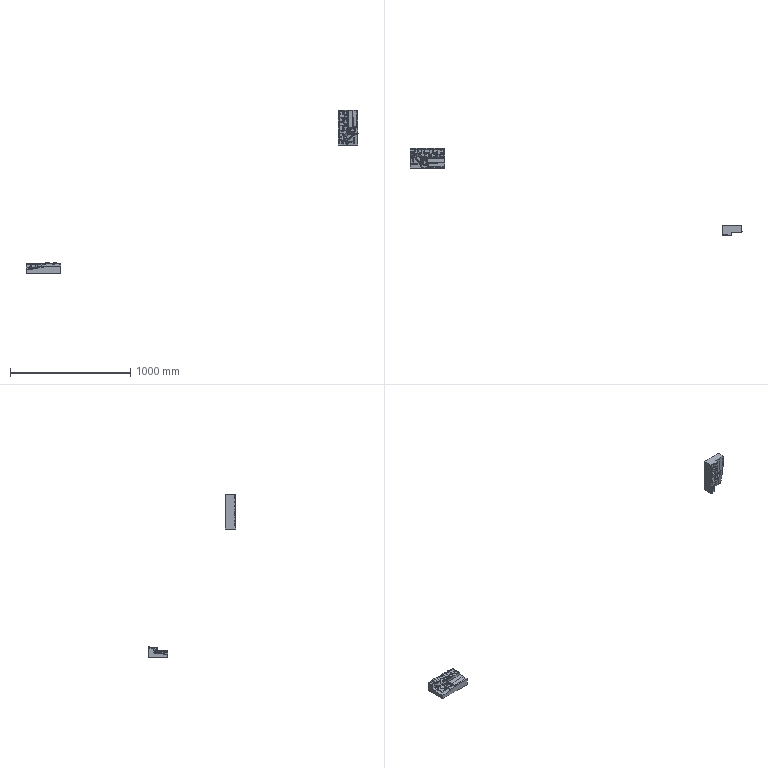NC program | NX | posted with a generic post | part box 2756 x 729.572 x 1353 mm
Lines 1 to 918 of 180527:
N10 G17 G21 G94 G90
(CAVITY_MILL , TOOL : D30R5)
N12 T00 M6
N14 G54
N16 G17 G0 G90 X96.082 Y-15. B0. C0. S3000 M3
N18 G43 Z10. H0
N20 Z-0.377
N22 G94 G1 Z-0.577 F2500.
N24 Y79.168
N26 X110.206
N28 G3 X111.586 Y83.525 R2.4
N30 G2 X109.837 Y84.788 R89.6
N32 G3 X108.189 Y85.332 R2.8
N34 G1 X81.958
N36 G3 X79.168 Y82.542 R2.8
N38 G1 Y81.958
N40 G3 X81.958 Y79.168 R2.8
N42 G1 X87.926
N44 G2 X90.753 Y77.997 R4.
N46 G1 X101.411 Y67.339
N48 G3 X104.239 Y66.168 R4.
N50 G1 X131.939
N52 G3 X133.985 Y67.016 R2.892
N54 G1 X136.507 Y69.538
N56 G2 X137.959 Y70.466 R4.
N58 G3 X137.288 Y80.049 R5.
N60 G1 X118.484 Y84.085
N62 G3 X112.546 Y80.246 R5.
N64 X116.386 Y74.308 R5.
N66 G1 X132.215 Y70.91
N68 G2 X133.844 Y69.965 R3.043
N70 G1 X136.049 Y67.5
N72 G3 X139.03 Y66.168 R4.
N74 G1 X216.344
N76 G3 X220.332 Y70.156 R4.
N78 G1 Y75.916
N80 G3 X216.903 Y79.864 R4.
N82 G2 X209.985 Y81.159 R78.298
N84 G3 X208.148 Y81.151 R4.
N86 G2 X187.561 Y78.856 R80.961
N88 X156.417 Y80.486 R433.583
N90 X114.741 Y97.439 R76.6
N92 G3 X112.232 Y98.332 R4.
N94 G1 X70.156
N96 G3 X66.168 Y94.344 R4.
N98 G1 Y70.156
N100 G3 X70.156 Y66.168 R4.
N102 G1 X87.926
N104 G2 X90.753 Y64.997 R4.
N106 G1 X101.411 Y54.339
N108 G3 X104.239 Y53.168 R4.
N110 G1 X229.343
N112 G3 X233.332 Y57.157 R4.
N114 G1 Y88.099
N116 G3 X229.361 Y92.088 R4.
N118 G1 X227.394 Y92.097
N120 G2 X210.104 Y94.552 R65.298
N122 G3 X207.922 Y94.543 R4.
N124 G2 X187.78 Y91.855 R67.961
N126 X157.563 Y93.435 R420.583
N128 X119.802 Y110.266 R63.6
N130 G3 X117.094 Y111.332 R4.
N132 G1 X57.157
N134 G3 X53.168 Y107.343 R4.
N136 G1 Y57.157
N138 G3 X57.157 Y53.168 R4.
N140 G1 X87.926
N142 G2 X90.753 Y51.997 R4.
N144 G1 X101.411 Y41.339
N146 G3 X104.239 Y40.168 R4.
N148 G1 X242.342
N150 G3 X246.332 Y44.158 R4.
N152 G1 Y101.503
N154 G3 X242.214 Y105.491 R4.
N156 G1 X229.605 Y105.087
N158 X227.469 Y105.096
N160 G2 X210.315 Y108.121 R52.298
N162 G3 X207.635 Y108.115 R4.
N164 G2 X187.999 Y104.853 R54.961
N166 X158.709 Y106.385 R407.583
N168 X125.493 Y123.01 R50.6
N170 G3 X122.532 Y124.332 R4.
N172 G1 X44.158
N174 G3 X40.168 Y120.342 R4.
N176 G1 Y44.158
N178 G3 X44.158 Y40.168 R4.
N180 G1 X87.926
N182 G2 X90.753 Y38.997 R4.
N184 G1 X101.411 Y28.339
N186 G3 X104.239 Y27.168 R4.
N188 G1 X255.342
N190 G3 X259.332 Y31.159 R4.
N192 G1 Y114.93
N194 G3 X255.092 Y118.914 R4.
N196 G1 X254.963 Y118.906
N198 X229.426 Y118.088
N200 X227.547 Y118.096
N202 G2 X210.703 Y122.031 R39.298
N204 G3 X207.234 Y122.033 R4.
N206 G2 X188.218 Y117.851 R41.961
N208 X159.854 Y119.334 R394.583
N210 X132.11 Y135.595 R37.6
N212 G3 X128.821 Y137.332 R4.
N214 G1 X31.159
N216 G3 X27.168 Y133.341 R4.
N218 G1 Y31.159
N220 G3 X31.159 Y27.168 R4.
N222 G1 X87.927
N224 G2 X90.753 Y25.997 R4.
N226 G1 X101.411 Y15.339
N228 G3 X104.239 Y14.168 R4.
N230 G1 X268.34
N232 G3 X272.332 Y18.16 R4.
N234 G1 Y131.544
N236 G3 X266.405 Y135.041 R4.
N238 G2 X255.95 Y131.993 R24.829
N240 G1 X254.348 Y131.893
N242 X229.246 Y131.089
N244 X227.629 Y131.096
N246 G2 X211.478 Y136.81 R26.298
N248 G3 X206.519 Y136.815 R4.
N250 G2 X203.506 Y134.763 R25.432
N252 X188.44 Y130.849 R28.961
N254 X161. Y132.284 R381.583
N256 X140.268 Y147.802 R24.6
N258 G3 X136.556 Y150.332 R4.
N260 G1 X18.16
N262 G3 X14.168 Y146.34 R4.
N264 G1 Y18.16
N266 G3 X18.16 Y14.168 R4.
N268 G1 X87.927
N270 G2 X90.753 Y12.997 R4.
N272 G1 X101.411 Y2.339
N274 G3 X104.239 Y1.168 R4.
N276 G1 X285.325
N278 X285.332 Y1.175
N280 Y163.325
N282 X285.325 Y163.332
N284 X277.317
N286 G3 X276.312 Y162.544 R1.035
N288 G1 X276.257 Y162.322
N290 G2 X274.203 Y159.827 R3.729
N292 G3 X271.408 Y156.302 R5.
N294 G1 X268.168 Y140.633
N296 G3 X272.052 Y134.724 R5.
N298 X277.961 Y138.608 R5.
N300 G1 X281.201 Y154.277
N302 G3 X279.47 Y159.159 R5.
N304 G2 X278.677 Y160.628 R2.198
N306 G1 X278.504 Y162.264
N308 G3 X277.317 Y163.332 R1.194
N310 G1 X267.447
N312 G3 X266.276 Y160.701 R4.
N314 G1 X265.962 Y154.284
N316 G2 X255.137 Y144.967 R11.829
N318 G1 X253.734 Y144.88
N320 X229.066 Y144.09
N322 X227.719 Y144.096
N324 G2 X214.917 Y154.284 R13.298
N326 G1 X214.732 Y155.628
N328 X214.716 Y160.518
N330 G3 X213.54 Y163.332 R4.
N332 G1 X204.354
N334 G3 X203.179 Y160.506 R4.
N336 G1 X203.178 Y156.971
N338 X203.157 Y156.337
N340 G2 X196.976 Y146.004 R12.432
N342 X188.663 Y143.847 R15.961
N344 X162.146 Y145.233 R368.583
N346 X151.57 Y156.571 R11.6
N348 G3 X151.615 Y157.164 R4.
N350 G1 Y158.315
N352 X151.6 Y160.531
N354 G3 X150.425 Y163.332 R4.
N356 G1 X1.175
N358 X1.168 Y163.325
N360 Y1.175
N362 X1.175 Y1.168
N364 X111.082
N366 Y-15.
N368 Z-0.377
N370 G0 Z0.3
N372 X98.438
N374 Z-0.954
N376 G1 Z-1.154
N378 Y0.305
N380 X100.31 Y78.305
N382 X100.349 Y78.304
N384 X108.571
N386 G3 X109.952 Y82.661 R2.4
N388 G2 X107.161 Y84.706 R92.093
N390 G3 X103.374 Y84.762 R3.2
N392 G2 X99.865 Y82.366 R91.256
N394 G3 X98.841 Y78.859 R2.8
N396 G1 X103.939 Y67.648
N398 G3 X107.58 Y65.304 R4.
N400 G1 X130.088
N402 G3 X132.123 Y66.147 R2.881
N404 G1 X134.632 Y68.651
N406 G2 X136.094 Y69.581 R4.
N408 G3 X135.457 Y79.167 R5.
N410 G1 X116.864 Y83.222
N412 G3 X110.914 Y79.402 R5.
N414 X114.733 Y73.451 R5.
N416 G1 X130.365 Y70.042
N418 G2 X131.982 Y69.099 R3.036
N420 G1 X134.179 Y66.64
N422 G3 X137.162 Y65.304 R4.
N424 G1 X217.208
N426 G3 X221.196 Y69.292 R4.
N428 G1 Y74.929
N430 G3 X217.713 Y78.883 R4.
N432 G2 X209.881 Y80.277 R80.509
N434 G3 X208.094 Y80.272 R4.
N436 G2 X187.608 Y78.062 R83.589
N438 X158.872 Y78.903 R1188.078
N440 G1 X155.904 Y79.168
N442 G2 X111.137 Y98.224 R79.093
N444 G3 X108.536 Y99.196 R4.
N446 G1 X102.191
N448 G3 X99.683 Y98.301 R4.
N450 G2 X68.363 Y82.795 R78.256
N452 G3 X65.305 Y78.92 R4.
N454 G1 X65.304 Y76.486
N456 G3 X66.287 Y74.411 R2.683
N458 G1 X69.002 Y72.189
N460 G2 X69.699 Y71.452 R4.
N462 G3 X74.683 Y69.488 R5.
N464 G1 X94.402 Y73.281
N466 G3 X98.368 Y79.135 R5.
N468 X92.513 Y83.101 R5.
N470 G1 X72.794 Y79.308
N472 G3 X68.931 Y75.772 R5.
N474 G2 X68.304 Y74.703 R2.48
N476 G1 X66.469 Y72.861
N478 G3 X65.304 Y70.04 R4.
N480 G1 Y69.292
N482 G3 X69.292 Y65.304 R4.
N484 G1 X90.282
N486 G2 X93.109 Y64.134 R4.
N488 G1 X103.766 Y53.476
N490 G3 X106.595 Y52.304 R4.
N492 G1 X230.207
N494 G3 X234.196 Y56.293 R4.
N496 G1 Y87.275
N498 G3 X230.148 Y91.263 R4.
N500 G1 X228.885 Y91.245
N502 G2 X210.014 Y93.647 R67.509
N504 G3 X207.904 Y93.643 R4.
N506 G2 X187.817 Y91.06 R70.589
N508 X159.716 Y91.88 R1175.078
N510 G1 X157.07 Y92.115
N512 G2 X116.428 Y111.042 R66.093
N514 G3 X113.629 Y112.196 R4.
N516 G1 X97.331
N518 G3 X94.627 Y111.132 R4.
N520 G2 X55.939 Y93.908 R65.256
N522 G3 X52.305 Y89.936 R4.
N524 G1 X52.304 Y56.293
N526 G3 X56.293 Y52.304 R4.
N528 G1 X90.282
N530 G2 X93.109 Y51.134 R4.
N532 G1 X103.766 Y40.476
N534 G3 X106.595 Y39.304 R4.
N536 G1 X243.206 Y39.305
N538 G3 X247.196 Y43.294 R4.
N540 G1 Y100.468
N542 G3 X243.147 Y104.457 R4.
N544 G1 X228.693 Y104.243
N546 G2 X210.234 Y107.176 R54.509
N548 G3 X207.66 Y107.174 R4.
N550 G2 X188.026 Y104.058 R57.589
N552 X160.558 Y104.856 R1162.078
N554 G1 X158.236 Y105.063
N556 G2 X122.356 Y123.778 R53.093
N558 G3 X119.312 Y125.196 R4.
N560 G1 X91.91
N562 G3 X88.959 Y123.885 R4.
N564 G2 X49.104 Y106.664 R52.256
N566 X43.558 Y106.724 R50.259
N568 G3 X39.305 Y102.743 R4.
N570 G1 X39.304 Y43.294
N572 G3 X43.294 Y39.304 R4.
N574 G1 X90.282
N576 G2 X93.109 Y38.134 R4.
N578 G1 X103.766 Y27.476
N580 G3 X106.595 Y26.304 R4.
N582 G1 X256.206 Y26.305
N584 G3 X260.196 Y30.295 R4.
N586 G1 Y113.805
N588 G3 X255.958 Y117.788 R4.
N590 G1 X254.465 Y117.695
N592 X248.763 Y117.541
N594 X228.501 Y117.242
N596 G2 X210.614 Y121.003 R41.509
N598 G3 X207.321 Y121.01 R4.
N600 G2 X188.235 Y117.057 R44.589
N602 X161.399 Y117.833 R1149.078
N604 G1 X159.396 Y118.011
N606 G2 X129.396 Y136.069 R40.093
N608 G1 X129.212 Y136.356
N610 G3 X125.855 Y138.196 R4.
N612 G1 X85.669
N614 G3 X82.401 Y136.489 R4.
N616 G2 X48.948 Y119.672 R39.256
N618 X31.903 Y122.757 R37.259
N620 G3 X26.305 Y119.1 R4.
N622 G1 X26.304 Y30.295
N624 G3 X30.295 Y26.304 R4.
N626 G1 X90.282
N628 G2 X93.109 Y25.134 R4.
N630 G1 X103.766 Y14.476
N632 G3 X106.595 Y13.305 R4.
N634 G1 X269.205
N636 G3 X273.196 Y17.296 R4.
N638 G1 Y130.415
N640 G3 X267.314 Y133.935 R4.
N642 G2 X256.995 Y130.878 R26.549
N644 G1 X253.886 Y130.684
N646 X248.492 Y130.539
N648 X228.309 Y130.241
N650 G2 X211.309 Y135.554 R28.509
N652 G3 X206.665 Y135.549 R4.
N654 G2 X203.193 Y133.443 R26.22
N656 X188.45 Y130.055 R31.589
N658 X162.238 Y130.809 R1136.078
N660 G1 X160.558 Y130.959
N662 G2 X140.291 Y143.161 R27.093
N664 X137.683 Y148.505 R24.237
N666 G3 X133.912 Y151.196 R4.
N668 G1 X78.066
N670 G3 X74.39 Y148.752 R4.
N672 G2 X49.006 Y132.679 R26.256
N674 G3 X48.569 Y132.673 R4.
N676 G2 X24.084 Y148.573 R24.259
N678 G3 X20.338 Y151.196 R4.
N680 G1 X17.296
N682 G3 X13.305 Y147.204 R4.
N684 G1 Y137.598
N686 G3 X14.313 Y135.488 R2.712
N688 G1 X16.734 Y133.534
N690 G2 X17.915 Y131.957 R4.
N692 G1 X20.798 Y125.016
N694 G3 X27.333 Y122.316 R5.
N696 X30.033 Y128.851 R5.
N698 G1 X26.081 Y138.366
N700 G3 X16.489 Y136.958 R5.
N702 G2 X15.892 Y135.616 R2.355
N704 G1 X14.302 Y133.862
N706 G3 X13.305 Y131.274 R3.854
N708 G1 Y17.296
N710 G3 X17.296 Y13.305 R4.
N712 G1 X90.282
N714 G2 X93.109 Y12.134 R4.
N716 G1 X103.766 Y1.476
N718 G3 X106.595 Y0.305 R4.
N720 G1 X284.031
N722 G3 X286.196 Y2.469 R4.
N724 G1 Y150.989
N726 G3 X285.2 Y152.257 R1.305
N728 G1 X284.428 Y152.445
N730 G2 X281.821 Y154.502 R4.
N732 G3 X272.527 Y153.444 R5.
N734 G1 X269.044 Y139.688
N736 G3 X272.663 Y133.614 R5.
N738 X278.738 Y137.234 R5.
N740 G1 X281.298 Y147.345
N742 G2 X283.485 Y149.326 R2.665
N744 G1 X284.954 Y149.547
N746 G3 X286.196 Y150.989 R1.458
N748 G1 Y162.031
N750 G3 X284.031 Y164.196 R4.
N752 G1 X270.638
N754 G3 X268.169 Y160.516 R4.
N756 G1 X268.156 Y155.628
N758 X267.971 Y154.284
N760 G2 X256.001 Y143.841 R13.549
N762 G1 X253.308 Y143.674
N764 X248.22 Y143.536
N766 X228.117 Y143.239
N768 G2 X217.129 Y147.577 R15.509
N770 X213.318 Y156.527 R12.444
N772 G1 X213.314 Y160.509
N774 G3 X210.845 Y164.196 R4.
N776 G1 X206.744
N778 G3 X204.593 Y160.905 R3.6
N780 G1 X204.595 Y156.971
N782 X204.591 Y156.678
N784 G2 X197.332 Y145.047 R13.22
N786 X188.663 Y143.053 R18.589
N788 X163.075 Y143.786 R1123.078
N790 G1 X162.402 Y143.846
N792 X161.728 Y143.906
N794 G2 X151.186 Y150.254 R14.093
N796 X149.367 Y156.381 R11.237
N798 G1 X149.366 Y160.506
N800 G3 X146.896 Y164.196 R4.
N802 G1 X65.7
N804 G3 X63.231 Y160.505 R4.
N806 G1 Y156.599
N808 G2 X49.011 Y145.704 R13.256
N810 G3 X48.2 Y145.692 R4.
N812 G2 X35.805 Y154.842 R11.259
N814 G1 X35.785 Y154.954
N816 X35.789 Y160.903
N818 G3 X33.638 Y164.196 R3.6
N820 G1 X2.469
N822 G3 X0.305 Y162.031 R4.
N824 G1 Y2.469
N826 G3 X2.469 Y0.305 R4.
N828 G1 X113.438
N830 Y-15.
N832 Z-0.954
N834 G0 Z-0.277
N836 X109.138
N838 Z-1.532
N840 G1 Z-1.732
N842 Y0.
N844 X109.902 Y78.
N846 X109.904
N848 X112.501
N850 G3 X112.924 Y79.476 R0.8
N852 G2 X111.658 Y80.279 R95.628
N854 G3 X110.812 Y80.286 R0.8
N856 G2 X109.494 Y79.484 R90.266
N858 G3 X109.138 Y78.587 R0.8
N860 G1 X114.561 Y67.271
N862 G3 X118.168 Y65. R4.
N864 G1 X128.596
N866 G3 X130.652 Y65.853 R2.905
N868 G1 X133.188 Y68.396
N870 G2 X134.629 Y69.321 R4.
N872 G3 X133.923 Y78.902 R5.
N874 G1 X119.29 Y81.989
N876 G3 X113.365 Y78.128 R5.
N878 X117.225 Y72.204 R5.
N880 G1 X128.869 Y69.748
N882 G2 X130.511 Y68.799 R3.05
N884 G1 X132.725 Y66.33
N886 G3 X135.704 Y65. R4.
N888 G1 X217.512
N890 G3 X221.5 Y68.988 R4.
N892 G1 Y74.267
N894 G3 X218. Y78.223 R4.
N896 G2 X209.849 Y79.639 R82.863
N898 G3 X208.097 Y79.635 R4.
N900 G2 X187.626 Y77.489 R84.885
N902 G1 X184.841 Y77.527
N904 X162.695 Y77.993
N906 X161.16 Y78.043
N908 G2 X118.109 Y91.591 R82.628
N910 X113.74 Y94.682 R77.9
N912 G3 X108.971 Y94.722 R4.
N914 G2 X91.919 Y85.247 R77.266
N916 X68.621 Y79.64 R83.261
N918 G3 X65. Y75.671 R4.
N920 G1 Y68.988
N922 G3 X68.988 Y65. R4.
N924 G1 X85.903
N926 G3 X88.191 Y66.015 R3.085
N928 G1 X90.517 Y68.587
N930 G2 X92.721 Y69.829 R4.
N932 G1 X105.086 Y72.226
N934 G3 X109.043 Y78.086 R5.
N936 X103.183 Y82.043 R5.
N938 G1 X87.458 Y78.995
N940 G3 X88.6 Y69.09 R5.
N942 G2 X90.308 Y68.778 R4.
N944 G1 X98.802 Y65.189
N946 G2 X99.639 Y64.709 R4.
N948 G1 X115.574 Y52.795
N950 G3 X117.966 Y52. R4.
N952 G1 X230.512
N954 G3 X234.5 Y55.988 R4.
N956 G1 Y86.63
N958 G3 X230.458 Y90.618 R4.
N960 G1 X229.291 Y90.602
N962 X227.152 Y90.613
N964 G2 X209.981 Y92.994 R69.863
N966 G3 X207.92 Y92.99 R4.
N968 G2 X187.827 Y90.487 R71.885
N970 G1 X185.067 Y90.525
N972 X163.04 Y90.989
N974 X161.551 Y91.037
N976 G2 X125.25 Y102.454 R69.628
N978 X114.502 Y111.306 R64.9
N980 G3 X111.663 Y112.5 R4.
N982 G1 X111.263
N984 G3 X108.467 Y111.349 R4.
N986 G2 X87.09 Y97.317 R64.266
N988 X64.595 Y92.382 R70.261
N990 G1 X62.355 Y92.288
N992 X55.905 Y92.154
N994 G3 X52. Y88.167 R4.
N996 G1 Y55.988
N998 G3 X55.988 Y52. R4.
N1000 G1 X100.983
N1002 G2 X103.809 Y50.829 R4.
N1004 G1 X114.467 Y40.172
N1006 G3 X117.295 Y39. R4.
N1008 G1 X243.511
N1010 G3 X247.5 Y42.989 R4.
N1012 G1 Y99.807
N1014 G3 X243.457 Y103.796 R4.
N1016 G1 X229.234 Y103.603
N1018 X227.277 Y103.612
N1020 G2 X210.189 Y106.497 R56.863
N1022 G3 X207.687 Y106.495 R4.
N1024 G2 X188.03 Y103.486 R58.885
N1026 G1 X185.293 Y103.523
N1028 X163.386 Y103.985
N1030 X161.939 Y104.031
N1032 G2 X132.39 Y113.317 R56.628
N1034 X120.563 Y124.026 R51.9
N1036 G3 X117.473 Y125.5 R4.
N1038 G1 X105.576
N1040 G3 X102.527 Y124.077 R4.
N1042 G2 X82.261 Y109.387 R51.266
N1044 X63.981 Y105.368 R57.261
N1046 G1 X61.947 Y105.282
N1048 X48.166 Y104.997
N1050 G2 X43.241 Y105.091 R55.915
N1052 G3 X39. Y101.11 R4.
N1054 G1 Y42.989
N1056 G3 X42.989 Y39. R4.
N1058 G1 X100.982
N1060 G2 X103.809 Y37.829 R4.
N1062 G1 X114.467 Y27.172
N1064 G3 X117.295 Y26. R4.
N1066 G1 X256.51
N1068 G3 X260.5 Y29.99 R4.
N1070 G1 Y113.029
N1072 G3 X256.31 Y117.015 R4.
N1074 G2 X255.367 Y116.978 R42.925
N1076 G1 X253.822 Y116.938
N1078 X229.178 Y116.603
N1080 X227.409 Y116.612
N1082 G2 X210.532 Y120.273 R43.863
N1084 G3 X207.357 Y120.276 R4.
N1086 G2 X188.236 Y116.484 R45.885
N1088 G1 X185.518 Y116.521
N1090 X163.731 Y116.98
N1092 X162.324 Y117.025
N1094 G2 X139.531 Y124.181 R43.628
N1096 X127.599 Y136.577 R38.9
N1098 G3 X124.191 Y138.5 R4.
N1100 G1 X98.996
N1102 G3 X95.625 Y136.636 R4.
N1104 G2 X77.432 Y121.457 R38.266
N1106 X63.36 Y118.353 R44.261
N1108 G1 X61.538 Y118.277
N1110 X47.868 Y117.993
N1112 G2 X31.421 Y120.821 R42.915
N1114 G3 X26. Y117.092 R4.
N1116 G1 Y29.99
N1118 G3 X29.99 Y26. R4.
N1120 G1 X100.983
N1122 G2 X103.809 Y24.829 R4.
N1124 G1 X114.467 Y14.172
N1126 G3 X117.295 Y13. R4.
N1128 G1 X269.508
N1130 G3 X273.5 Y16.992 R4.
N1132 G1 Y129.635
N1134 G3 X267.698 Y133.198 R4.
N1136 G2 X255.013 Y129.973 R29.925
N1138 G1 X253.565 Y129.935
N1140 X229.122 Y129.604
N1142 X227.554 Y129.611
N1144 G2 X211.499 Y134.443 R30.863
N1146 X211.159 Y134.664 R26.394
N1148 G3 X206.765 Y134.661 R4.
N1150 G2 X204.885 Y133.526 R26.556
N1152 X188.446 Y129.482 R32.885
N1154 G1 X185.744 Y129.519
N1156 X164.076 Y129.976
N1158 X162.704 Y130.02
N1160 G2 X146.672 Y135.044 R30.628
N1162 X136.248 Y148.736 R25.9
N1164 G3 X132.452 Y151.5 R4.
N1166 G1 X90.896
N1168 G3 X87.123 Y148.804 R4.
N1170 G2 X72.603 Y133.527 R25.266
N1172 X62.725 Y131.338 R31.261
N1174 G1 X61.13 Y131.271
N1176 X47.565 Y130.99
N1178 G2 X29.225 Y136.669 R29.915
N1180 X20.292 Y149.006 R24.428
N1182 G3 X16.874 Y151.5 R3.6
N1184 G1 X16.592
N1186 G3 X13. Y147.908 R3.6
N1188 G1 Y16.992
N1190 G3 X16.992 Y13. R4.
N1192 G1 X100.983
N1194 G2 X103.809 Y11.829 R4.
N1196 G1 X114.467 Y1.172
N1198 G3 X117.295 Y0. R4.
N1200 G1 X282.505
N1202 G3 X286.5 Y3.995 R4.
N1204 G1 Y148.788
N1206 G3 X285.548 Y150.011 R1.261
N1208 G1 X284.924 Y150.168
N1210 G2 X282.302 Y152.309 R4.
N1212 G3 X272.983 Y151.491 R5.
N1214 G1 X269.468 Y138.968
N1216 G3 X272.93 Y132.803 R5.
N1218 X279.096 Y136.265 R5.
N1220 G1 X281.621 Y145.261
N1222 G2 X283.788 Y147.156 R2.633
N1224 G1 X285.262 Y147.364
N1226 G3 X286.5 Y148.788 R1.438
N1228 G1 Y160.505
N1230 G3 X282.505 Y164.5 R4.
N1232 G1 X273.394
N1234 G3 X269.399 Y160.507 R4.
N1236 G1 X269.397 Y156.971
N1238 G2 X264.082 Y146.174 R13.143
N1240 X254.654 Y142.968 R16.925
N1242 G1 X253.308 Y142.933
N1244 X229.066 Y142.604
N1246 X227.719 Y142.611
N1248 G2 X218.486 Y145.406 R17.863
N1250 X212.295 Y156.359 R13.394
N1252 G1 X212.279 Y156.971
N1254 Y161.306
N1256 G3 X209.085 Y164.5 R3.2
N1258 G1 X208.873
N1260 G3 X205.679 Y161.304 R3.2
N1262 G1 X205.681 Y156.971
N1264 X205.67 Y156.496
N1266 G2 X198.635 Y144.925 R13.556
N1268 X188.663 Y142.481 R19.885
N1270 G1 X185.97 Y142.517
N1272 X164.422 Y142.972
N1274 X163.075 Y143.015
N1276 G2 X153.812 Y145.907 R17.628
N1278 X148.003 Y156.317 R12.9
N1280 G1 X147.984 Y156.971
N1282 X147.985 Y160.905
N1284 G3 X144.39 Y164.5 R3.6
N1286 G1 X78.996
N1288 G3 X75.402 Y160.826 R3.6
N1290 G1 X75.481 Y157.256
N1292 G2 X67.774 Y145.597 R12.266
N1294 X62.068 Y144.322 R18.261
N1296 G1 X60.721 Y144.265
N1298 X47.254 Y143.986
N1300 G2 X36.852 Y147.197 R16.915
N1302 X32.134 Y156.135 R11.428
N1304 G1 X32.111 Y156.971
N1306 X32.115 Y160.901
N1308 G3 X28.521 Y164.5 R3.6
N1310 G1 X3.995
N1312 G3 X0. Y160.505 R4.
N1314 G1 Y3.995
N1316 G3 X3.995 Y0. R4.
N1318 G1 X124.138
N1320 Y-15.
N1322 Z-1.532
N1324 G0 Z-0.854
N1326 X143.25
N1328 Z-2.109
N1330 G1 Z-2.309
N1332 Y65.
N1334 X217.512
N1336 G3 X221.5 Y68.988 R4.
N1338 G1 Y73.802
N1340 G3 X217.986 Y77.76 R4.
N1342 G2 X209.804 Y79.15 R84.079
N1344 G3 X208.107 Y79.151 R4.
N1346 G2 X188.006 Y77.085 R89.159
N1348 X161.74 Y77.474 R1970.402
N1350 X135.105 Y82.351 R84.447
N1352 G3 X132.815 Y82.462 R4.
N1354 G2 X98.315 Y81.769 R77.237
N1356 X91.823 Y83.196 R77.146
N1358 G3 X89.496 Y83.106 R4.
N1360 G2 X68.655 Y78.655 R84.131
N1362 G3 X65. Y74.682 R4.
N1364 G1 Y68.988
N1366 G3 X68.988 Y65. R4.
N1368 G1 X135.094
N1370 G2 X137.921 Y63.829 R4.
N1372 G1 X148.578 Y53.172
N1374 G3 X151.407 Y52. R4.
N1376 G1 X230.511
N1378 G3 X234.5 Y55.989 R4.
N1380 G1 Y86.186
N1382 G3 X230.471 Y90.175 R4.
N1384 G1 X229.224 Y90.162
N1386 X227.344 Y90.17
N1388 G2 X209.97 Y92.48 R71.079
N1390 G3 X207.981 Y92.483 R4.
N1392 G2 X207.324 Y92.317 R69.062
N1394 X188.132 Y90.085 R76.159
N1396 X162.01 Y90.471 R1957.402
N1398 X135.949 Y95.956 R71.447
N1400 G3 X133.238 Y96.08 R4.
N1402 G2 X100.761 Y94.539 R64.237
N1404 X91.531 Y96.84 R64.146
N1406 G3 X88.775 Y96.739 R4.
N1408 G2 X63.267 Y91.381 R71.131
N1410 G1 X61.704 Y91.345
N1412 X55.932 Y91.263
N1414 G3 X52. Y87.275 R4.
N1416 G1 Y55.989
N1418 G3 X55.989 Y52. R4.
N1420 G1 X135.094
N1422 G2 X137.92 Y50.829 R4.
N1424 G1 X148.578 Y40.172
N1426 G3 X151.407 Y39. R4.
N1428 G1 X243.511
N1430 G3 X247.5 Y42.989 R4.
N1432 G1 Y99.317
N1434 G3 X243.47 Y103.306 R4.
N1436 G1 X229.185 Y103.162
N1438 X227.429 Y103.169
N1440 G2 X210.197 Y105.948 R58.079
N1442 G3 X207.778 Y105.95 R4.
N1444 G2 X204.196 Y104.935 R56.062
N1446 X188.26 Y103.084 R63.159
N1448 X162.278 Y103.468 R1944.402
N1450 X136.846 Y109.856 R58.447
N1452 G3 X133.526 Y109.993 R4.
N1454 G2 X103.207 Y107.31 R51.237
N1456 X91.379 Y110.788 R51.146
N1458 G3 X88.002 Y110.681 R4.
N1460 G2 X62.966 Y104.378 R58.131
N1462 G1 X61.458 Y104.342
N1464 X49.408 Y104.171
N1466 X48.072 Y104.135
N1468 G2 X43.236 Y104.241 R60.832
N1470 G3 X39. Y100.259 R4.
N1472 G1 Y42.989
N1474 G3 X42.989 Y39. R4.
N1476 G1 X135.095
N1478 G2 X137.921 Y37.829 R4.
N1480 G1 X148.578 Y27.172
N1482 G3 X151.407 Y26. R4.
N1484 G1 X256.51
N1486 G3 X260.5 Y29.99 R4.
N1488 G1 Y112.49
N1490 G3 X256.325 Y116.476 R4.
N1492 G2 X255.157 Y116.437 R44.134
N1494 G1 X253.68 Y116.41
N1496 X229.145 Y116.163
N1498 X227.518 Y116.169
N1500 G2 X210.522 Y119.674 R45.079
N1502 G3 X207.44 Y119.671 R4.
N1504 G2 X201.069 Y117.553 R43.062
N1506 X188.39 Y116.084 R50.159
N1508 X162.546 Y116.465 R1931.402
N1510 X140.533 Y122.65 R45.447
N1512 X137.876 Y124.346 R39.513
N1514 G3 X133.567 Y124.502 R4.
N1516 G2 X105.653 Y120.083 R38.237
N1518 X91.484 Y125.36 R38.146
N1520 G3 X87.099 Y125.241 R4.
N1522 G2 X84.855 Y123.787 R38.327
N1524 X62.665 Y117.375 R45.131
N1526 G1 X61.213 Y117.34
N1528 X49.139 Y117.169
N1530 X47.786 Y117.132
N1532 G2 X31.302 Y119.77 R47.832
N1534 G3 X26. Y115.997 R4.
N1536 G1 Y29.99
N1538 G3 X29.99 Y26. R4.
N1540 G1 X135.095
N1542 G2 X137.92 Y24.83 R4.
N1544 G1 X148.578 Y14.172
N1546 G3 X151.407 Y13. R4.
N1548 G1 X269.508
N1550 G3 X273.5 Y16.992 R4.
N1552 G1 Y128.902
N1554 G3 X267.775 Y132.502 R4.
N1556 G2 X254.907 Y129.435 R31.134
N1558 G1 X253.494 Y129.409
N1560 X229.106 Y129.163
N1562 X227.613 Y129.169
N1564 G2 X211.801 Y133.531 R32.079
N1566 X211.064 Y133.977 R26.847
N1568 G3 X206.812 Y133.965 R4.
N1570 G2 X197.941 Y130.171 R30.062
N1572 X188.524 Y129.083 R37.159
N1574 X162.812 Y129.462 R1918.402
N1576 X147.084 Y133.879 R32.447
N1578 X139.358 Y140.708 R26.513
N1580 G3 X133.16 Y140.897 R4.
N1582 G2 X108.101 Y132.861 R25.237
N1584 X92.026 Y141.995 R25.146
N1586 G3 X85.678 Y141.83 R4.
N1588 G2 X78.17 Y134.937 R25.327
N1590 X62.366 Y130.371 R32.131
N1592 G1 X60.967 Y130.338
N1594 X48.87 Y130.166
N1596 X47.511 Y130.129
N1598 G2 X31.93 Y133.547 R34.832
N1600 X18.251 Y149.764 R25.833
N1602 G3 X15.952 Y151.5 R2.4
N1604 G1 X15.393
N1606 G3 X13. Y149.107 R2.4
N1608 G1 Y16.992
N1610 G3 X16.992 Y13. R4.
N1612 G1 X135.095
N1614 G2 X137.92 Y11.83 R4.
N1616 G1 X148.578 Y1.172
N1618 G3 X151.407 Y0. R4.
N1620 G1 X282.505
N1622 G3 X286.5 Y3.995 R4.
N1624 G1 Y146.969
N1626 G3 X285.588 Y148.149 R1.22
N1628 G1 X285.105 Y148.275
N1630 G2 X282.469 Y150.498 R4.
N1632 G3 X273.133 Y149.911 R5.
N1634 G1 X269.561 Y138.304
N1636 G3 X272.868 Y132.054 R5.
N1638 X279.118 Y135.362 R5.
N1640 G1 X281.639 Y143.552
N1642 G2 X283.787 Y145.366 R2.603
N1644 G1 X285.265 Y145.561
N1646 G3 X286.5 Y146.969 R1.42
N1648 G1 Y160.505
N1650 G3 X282.505 Y164.5 R4.
N1652 G1 X274.321
N1654 G3 X270.326 Y160.505 R4.
N1656 G1 X270.325 Y156.971
N1658 X270.316 Y156.455
N1660 G2 X264.116 Y145.324 R13.544
N1662 X254.654 Y142.433 R18.134
N1664 G1 X253.308 Y142.408
N1666 X229.066 Y142.163
N1668 X227.719 Y142.169
N1670 G2 X218.347 Y144.763 R19.079
N1672 X211.477 Y156.373 R13.847
N1674 G1 X211.462 Y156.971
N1676 X211.461 Y162.106
N1678 G3 X209.066 Y164.5 R2.4
N1680 G1 X208.949
N1682 G3 X206.554 Y162.104 R2.4
N1684 G1 X206.558 Y156.733
N1686 G2 X201.769 Y146.359 R13.613
N1688 X194.814 Y142.789 R17.062
N1690 X188.663 Y142.082 R24.159
N1692 X163.075 Y142.46 R1905.402
N1694 X153.636 Y145.107 R19.447
N1696 X146.94 Y156.364 R13.513
N1698 G1 X146.921 Y156.971
N1700 Y160.905
N1702 G3 X143.327 Y164.5 R3.6
N1704 G1 X138.11
N1706 X138.029 Y164.504
N1708 X138.007 Y164.426
N1710 G2 X137.672 Y164.161 R0.39
N1712 G3 X133.234 Y160.29 R5.
N1714 G1 X130.596 Y148.702
N1716 G3 X134.361 Y142.717 R5.
N1718 X140.346 Y146.482 R5.
N1720 G1 X142.985 Y158.07
N1722 G3 X138.414 Y164.171 R5.
N1724 G2 X138.236 Y164.322 R0.195
N1726 G1 X138.215 Y164.416
N1728 X138.217 Y164.478
N1730 X138.169 Y164.516
N1732 X138.11 Y164.5
N1734 X130.12
N1736 G3 X126.125 Y160.562 R4.
N1738 G1 X126.045 Y154.945
N1740 G2 X110.841 Y145.578 R12.237
N1742 G3 X110.252 Y145.691 R4.
N1744 G2 X99.526 Y156.606 R12.146
N1746 G1 Y160.505
N1748 G3 X95.531 Y164.5 R4.
N1750 G1 X81.484
N1752 G3 X77.489 Y160.507 R4.
N1754 G1 X77.488 Y157.629
N1756 G3 X77.818 Y157.214 R0.425
N1758 G2 X78.944 Y156.164 R1.54
N1760 G3 X80.47 Y153.832 R5.
N1762 G1 X88.948 Y146.556
N1764 G3 X95.998 Y147.094 R5.
N1766 X95.46 Y154.145 R5.
N1768 G1 X86.982 Y161.42
N1770 G3 X78.847 Y158.721 R5.
N1772 G2 X78.257 Y158.137 R0.77
N1774 G1 X77.824 Y158.044
N1776 G3 X77.488 Y157.629 R0.425
N1778 G1 X77.487 Y156.971
N1780 X77.468 Y156.299
N1782 G2 X71.485 Y146.086 R12.327
N1784 X62.068 Y143.368 R19.131
N1786 G1 X60.721 Y143.336
N1788 X48.601 Y143.164
N1790 X47.254 Y143.127
N1792 G2 X37.549 Y145.27 R21.832
N1794 X30.269 Y156.443 R12.833
N1796 G1 X30.252 Y156.971
N1798 X30.254 Y160.904
N1800 G3 X26.66 Y164.5 R3.6
N1802 G1 X3.995
N1804 G3 X0. Y160.505 R4.
N1806 G1 Y3.995
N1808 G3 X3.995 Y0. R4.
N1810 G1 X158.25
N1812 Y-15.
N1814 Z-2.109
N1816 G0 Z-1.432
N1818 X143.25
N1820 Z-2.686
N1822 G1 Z-2.886
N1824 Y65.
N1826 X217.513
N1828 G3 X221.5 Y68.987 R4.
N1830 G1 Y73.472
N1832 G3 X217.976 Y77.431 R4.
N1834 G2 X209.839 Y78.774 R86.748